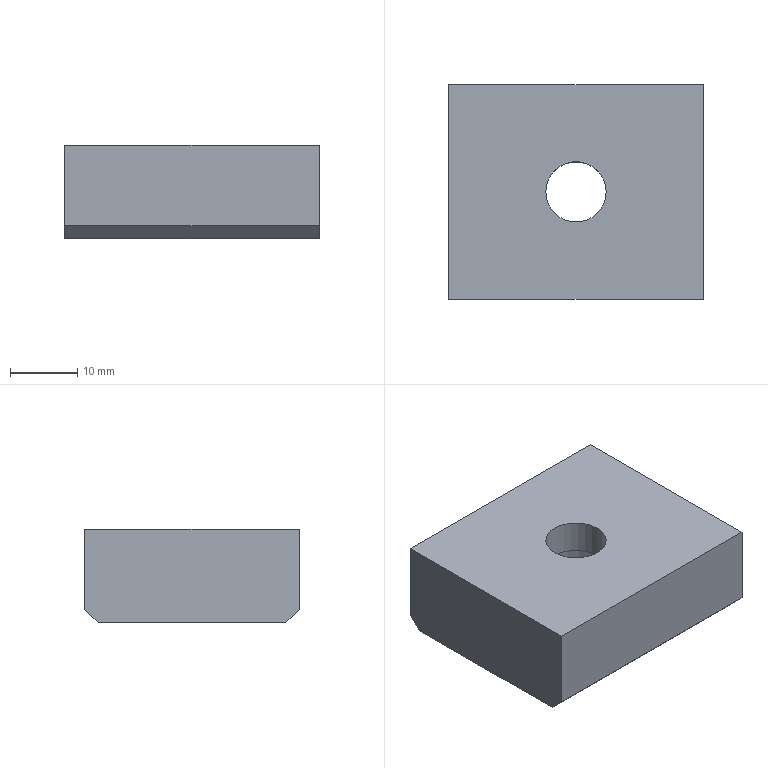Part | NX | features solid 2 | 1 solid | 11 faces | box 38 x 32 x 14 mm | volume 15168 mm3 | plane 9 | cylinder 2 | commonest cylinder face diameters 9 x1 14 x1
STEP:
#1=CARTESIAN_POINT('',(204.,-294.,102.));
#2=VERTEX_POINT('',#1);
#3=CARTESIAN_POINT('',(204.,-294.,114.));
#4=VERTEX_POINT('',#3);
#5=CARTESIAN_POINT('',(204.,-294.,100.));
#6=DIRECTION('',(0.,0.,1.));
#7=VECTOR('',#6,1000.);
#8=LINE('',#5,#7);
#9=EDGE_CURVE('',#2,#4,#8,.T.);
#10=ORIENTED_EDGE('',*,*,#9,.F.);
#11=CARTESIAN_POINT('',(166.,-294.,102.));
#12=VERTEX_POINT('',#11);
#13=CARTESIAN_POINT('',(160.,-294.,102.));
#14=DIRECTION('',(-1.,0.,0.));
#15=VECTOR('',#14,1000.);
#16=LINE('',#13,#15);
#17=EDGE_CURVE('',#2,#12,#16,.T.);
#18=ORIENTED_EDGE('',*,*,#17,.T.);
#19=CARTESIAN_POINT('',(166.,-294.,114.));
#20=VERTEX_POINT('',#19);
#21=CARTESIAN_POINT('',(166.,-294.,100.));
#22=DIRECTION('',(0.,0.,-1.));
#23=VECTOR('',#22,1000.);
#24=LINE('',#21,#23);
#25=EDGE_CURVE('',#12,#20,#24,.F.);
#26=ORIENTED_EDGE('',*,*,#25,.T.);
#27=CARTESIAN_POINT('',(160.,-294.,114.));
#28=DIRECTION('',(-1.,0.,0.));
#29=VECTOR('',#28,1000.);
#30=LINE('',#27,#29);
#31=EDGE_CURVE('',#20,#4,#30,.F.);
#32=ORIENTED_EDGE('',*,*,#31,.T.);
#33=EDGE_LOOP('',(#10,#18,#26,#32));
#34=FACE_BOUND('',#33,.T.);
#35=CARTESIAN_POINT('',(160.,-294.,100.));
#36=DIRECTION('',(0.,1.,0.));
#37=DIRECTION('',(1.,0.,0.));
#38=AXIS2_PLACEMENT_3D('',#35,#36,#37);
#39=PLANE('',#38);
#40=ADVANCED_FACE('',(#34),#39,.T.);
#41=ORIENTED_EDGE('',*,*,#25,.F.);
#42=CARTESIAN_POINT('',(166.,-296.,100.));
#43=VERTEX_POINT('',#42);
#44=CARTESIAN_POINT('',(166.,-298.,98.));
#45=DIRECTION('',(0.,-0.7071,-0.7071));
#46=VECTOR('',#45,1000.);
#47=LINE('',#44,#46);
#48=EDGE_CURVE('',#12,#43,#47,.T.);
#49=ORIENTED_EDGE('',*,*,#48,.T.);
#50=CARTESIAN_POINT('',(166.,-324.,100.));
#51=VERTEX_POINT('',#50);
#52=CARTESIAN_POINT('',(166.,-300.,100.));
#53=DIRECTION('',(0.,1.,0.));
#54=VECTOR('',#53,1000.);
#55=LINE('',#52,#54);
#56=EDGE_CURVE('',#43,#51,#55,.F.);
#57=ORIENTED_EDGE('',*,*,#56,.T.);
#58=CARTESIAN_POINT('',(166.,-326.,102.));
#59=VERTEX_POINT('',#58);
#60=CARTESIAN_POINT('',(166.,-312.,88.));
#61=DIRECTION('',(0.,0.7071,-0.7071));
#62=VECTOR('',#61,1000.);
#63=LINE('',#60,#62);
#64=EDGE_CURVE('',#51,#59,#63,.F.);
#65=ORIENTED_EDGE('',*,*,#64,.T.);
#66=CARTESIAN_POINT('',(166.,-326.,114.));
#67=VERTEX_POINT('',#66);
#68=CARTESIAN_POINT('',(166.,-326.,100.));
#69=DIRECTION('',(0.,0.,1.));
#70=VECTOR('',#69,1000.);
#71=LINE('',#68,#70);
#72=EDGE_CURVE('',#59,#67,#71,.T.);
#73=ORIENTED_EDGE('',*,*,#72,.T.);
#74=CARTESIAN_POINT('',(166.,-300.,114.));
#75=DIRECTION('',(0.,1.,0.));
#76=VECTOR('',#75,1000.);
#77=LINE('',#74,#76);
#78=EDGE_CURVE('',#20,#67,#77,.F.);
#79=ORIENTED_EDGE('',*,*,#78,.F.);
#80=EDGE_LOOP('',(#41,#49,#57,#65,#73,#79));
#81=FACE_BOUND('',#80,.T.);
#82=CARTESIAN_POINT('',(166.,-300.,100.));
#83=DIRECTION('',(1.,0.,0.));
#84=DIRECTION('',(0.,-1.,0.));
#85=AXIS2_PLACEMENT_3D('',#82,#83,#84);
#86=PLANE('',#85);
#87=ADVANCED_FACE('',(#81),#86,.F.);
#88=ORIENTED_EDGE('',*,*,#72,.F.);
#89=CARTESIAN_POINT('',(204.,-326.,102.));
#90=VERTEX_POINT('',#89);
#91=CARTESIAN_POINT('',(160.,-326.,102.));
#92=DIRECTION('',(-1.,0.,0.));
#93=VECTOR('',#92,1000.);
#94=LINE('',#91,#93);
#95=EDGE_CURVE('',#59,#90,#94,.F.);
#96=ORIENTED_EDGE('',*,*,#95,.T.);
#97=CARTESIAN_POINT('',(204.,-326.,114.));
#98=VERTEX_POINT('',#97);
#99=CARTESIAN_POINT('',(204.,-326.,100.));
#100=DIRECTION('',(0.,0.,-1.));
#101=VECTOR('',#100,1000.);
#102=LINE('',#99,#101);
#103=EDGE_CURVE('',#90,#98,#102,.F.);
#104=ORIENTED_EDGE('',*,*,#103,.T.);
#105=CARTESIAN_POINT('',(160.,-326.,114.));
#106=DIRECTION('',(-1.,0.,0.));
#107=VECTOR('',#106,1000.);
#108=LINE('',#105,#107);
#109=EDGE_CURVE('',#67,#98,#108,.F.);
#110=ORIENTED_EDGE('',*,*,#109,.F.);
#111=EDGE_LOOP('',(#88,#96,#104,#110));
#112=FACE_BOUND('',#111,.T.);
#113=CARTESIAN_POINT('',(160.,-326.,100.));
#114=DIRECTION('',(0.,1.,0.));
#115=DIRECTION('',(1.,0.,0.));
#116=AXIS2_PLACEMENT_3D('',#113,#114,#115);
#117=PLANE('',#116);
#118=ADVANCED_FACE('',(#112),#117,.F.);
#119=CARTESIAN_POINT('',(180.5,-310.,114.));
#120=VERTEX_POINT('',#119);
#121=CARTESIAN_POINT('',(185.,-310.,114.));
#122=DIRECTION('',(0.,0.,-1.));
#123=DIRECTION('',(-1.,0.,0.));
#124=AXIS2_PLACEMENT_3D('',#121,#122,#123);
#125=CIRCLE('',#124,4.5);
#126=EDGE_CURVE('',#120,#120,#125,.T.);
#127=ORIENTED_EDGE('',*,*,#126,.T.);
#128=EDGE_LOOP('',(#127));
#129=FACE_BOUND('',#128,.T.);
#130=ORIENTED_EDGE('',*,*,#109,.T.);
#131=CARTESIAN_POINT('',(204.,-300.,114.));
#132=DIRECTION('',(0.,-1.,0.));
#133=VECTOR('',#132,1000.);
#134=LINE('',#131,#133);
#135=EDGE_CURVE('',#4,#98,#134,.T.);
#136=ORIENTED_EDGE('',*,*,#135,.F.);
#137=ORIENTED_EDGE('',*,*,#31,.F.);
#138=ORIENTED_EDGE('',*,*,#78,.T.);
#139=EDGE_LOOP('',(#130,#136,#137,#138));
#140=FACE_BOUND('',#139,.T.);
#141=CARTESIAN_POINT('',(160.,-300.,114.));
#142=DIRECTION('',(0.,0.,-1.));
#143=DIRECTION('',(-1.,0.,0.));
#144=AXIS2_PLACEMENT_3D('',#141,#142,#143);
#145=PLANE('',#144);
#146=ADVANCED_FACE('',(#129,#140),#145,.F.);
#147=CARTESIAN_POINT('',(204.,-296.,100.));
#148=VERTEX_POINT('',#147);
#149=CARTESIAN_POINT('',(204.,-324.,100.));
#150=VERTEX_POINT('',#149);
#151=CARTESIAN_POINT('',(204.,-300.,100.));
#152=DIRECTION('',(0.,-1.,0.));
#153=VECTOR('',#152,1000.);
#154=LINE('',#151,#153);
#155=EDGE_CURVE('',#148,#150,#154,.T.);
#156=ORIENTED_EDGE('',*,*,#155,.F.);
#157=CARTESIAN_POINT('',(204.,-298.,98.));
#158=DIRECTION('',(0.,-0.7071,-0.7071));
#159=VECTOR('',#158,1000.);
#160=LINE('',#157,#159);
#161=EDGE_CURVE('',#148,#2,#160,.F.);
#162=ORIENTED_EDGE('',*,*,#161,.T.);
#163=ORIENTED_EDGE('',*,*,#9,.T.);
#164=ORIENTED_EDGE('',*,*,#135,.T.);
#165=ORIENTED_EDGE('',*,*,#103,.F.);
#166=CARTESIAN_POINT('',(204.,-312.,88.));
#167=DIRECTION('',(0.,0.7071,-0.7071));
#168=VECTOR('',#167,1000.);
#169=LINE('',#166,#168);
#170=EDGE_CURVE('',#90,#150,#169,.T.);
#171=ORIENTED_EDGE('',*,*,#170,.T.);
#172=EDGE_LOOP('',(#156,#162,#163,#164,#165,#171));
#173=FACE_BOUND('',#172,.T.);
#174=CARTESIAN_POINT('',(204.,-300.,100.));
#175=DIRECTION('',(1.,0.,0.));
#176=DIRECTION('',(0.,-1.,0.));
#177=AXIS2_PLACEMENT_3D('',#174,#175,#176);
#178=PLANE('',#177);
#179=ADVANCED_FACE('',(#173),#178,.T.);
#180=CARTESIAN_POINT('',(192.,-310.,100.));
#181=VERTEX_POINT('',#180);
#182=CARTESIAN_POINT('',(185.,-310.,100.));
#183=DIRECTION('',(0.,0.,1.));
#184=DIRECTION('',(1.,0.,0.));
#185=AXIS2_PLACEMENT_3D('',#182,#183,#184);
#186=CIRCLE('',#185,7.);
#187=EDGE_CURVE('',#181,#181,#186,.T.);
#188=ORIENTED_EDGE('',*,*,#187,.T.);
#189=EDGE_LOOP('',(#188));
#190=FACE_BOUND('',#189,.T.);
#191=ORIENTED_EDGE('',*,*,#56,.F.);
#192=CARTESIAN_POINT('',(160.,-296.,100.));
#193=DIRECTION('',(1.,0.,0.));
#194=VECTOR('',#193,1000.);
#195=LINE('',#192,#194);
#196=EDGE_CURVE('',#43,#148,#195,.T.);
#197=ORIENTED_EDGE('',*,*,#196,.T.);
#198=ORIENTED_EDGE('',*,*,#155,.T.);
#199=CARTESIAN_POINT('',(160.,-324.,100.));
#200=DIRECTION('',(-1.,0.,0.));
#201=VECTOR('',#200,1000.);
#202=LINE('',#199,#201);
#203=EDGE_CURVE('',#150,#51,#202,.T.);
#204=ORIENTED_EDGE('',*,*,#203,.T.);
#205=EDGE_LOOP('',(#191,#197,#198,#204));
#206=FACE_BOUND('',#205,.T.);
#207=CARTESIAN_POINT('',(160.,-300.,100.));
#208=DIRECTION('',(0.,0.,-1.));
#209=DIRECTION('',(-1.,0.,0.));
#210=AXIS2_PLACEMENT_3D('',#207,#208,#209);
#211=PLANE('',#210);
#212=ADVANCED_FACE('',(#190,#206),#211,.T.);
#213=ORIENTED_EDGE('',*,*,#48,.F.);
#214=ORIENTED_EDGE('',*,*,#17,.F.);
#215=ORIENTED_EDGE('',*,*,#161,.F.);
#216=ORIENTED_EDGE('',*,*,#196,.F.);
#217=EDGE_LOOP('',(#213,#214,#215,#216));
#218=FACE_BOUND('',#217,.T.);
#219=CARTESIAN_POINT('',(160.,-296.,100.));
#220=DIRECTION('',(0.,-0.7071,0.7071));
#221=DIRECTION('',(0.,-0.7071,-0.7071));
#222=AXIS2_PLACEMENT_3D('',#219,#220,#221);
#223=PLANE('',#222);
#224=ADVANCED_FACE('',(#218),#223,.F.);
#225=ORIENTED_EDGE('',*,*,#64,.F.);
#226=ORIENTED_EDGE('',*,*,#203,.F.);
#227=ORIENTED_EDGE('',*,*,#170,.F.);
#228=ORIENTED_EDGE('',*,*,#95,.F.);
#229=EDGE_LOOP('',(#225,#226,#227,#228));
#230=FACE_BOUND('',#229,.T.);
#231=CARTESIAN_POINT('',(160.,-326.,102.));
#232=DIRECTION('',(0.,-0.7071,-0.7071));
#233=DIRECTION('',(0.,0.7071,-0.7071));
#234=AXIS2_PLACEMENT_3D('',#231,#232,#233);
#235=PLANE('',#234);
#236=ADVANCED_FACE('',(#230),#235,.T.);
#237=ORIENTED_EDGE('',*,*,#187,.F.);
#238=EDGE_LOOP('',(#237));
#239=FACE_BOUND('',#238,.T.);
#240=CARTESIAN_POINT('',(192.,-310.,109.));
#241=VERTEX_POINT('',#240);
#242=CARTESIAN_POINT('',(185.,-310.,109.));
#243=DIRECTION('',(0.,0.,1.));
#244=DIRECTION('',(1.,0.,0.));
#245=AXIS2_PLACEMENT_3D('',#242,#243,#244);
#246=CIRCLE('',#245,7.);
#247=EDGE_CURVE('',#241,#241,#246,.T.);
#248=ORIENTED_EDGE('',*,*,#247,.T.);
#249=EDGE_LOOP('',(#248));
#250=FACE_BOUND('',#249,.T.);
#251=CARTESIAN_POINT('',(185.,-310.,100.));
#252=DIRECTION('',(0.,0.,1.));
#253=DIRECTION('',(1.,0.,0.));
#254=AXIS2_PLACEMENT_3D('',#251,#252,#253);
#255=CYLINDRICAL_SURFACE('',#254,7.);
#256=ADVANCED_FACE('',(#239,#250),#255,.F.);
#257=CARTESIAN_POINT('',(189.5,-310.,109.));
#258=VERTEX_POINT('',#257);
#259=CARTESIAN_POINT('',(185.,-310.,109.));
#260=DIRECTION('',(0.,0.,1.));
#261=DIRECTION('',(1.,0.,0.));
#262=AXIS2_PLACEMENT_3D('',#259,#260,#261);
#263=CIRCLE('',#262,4.5);
#264=EDGE_CURVE('',#258,#258,#263,.T.);
#265=ORIENTED_EDGE('',*,*,#264,.T.);
#266=EDGE_LOOP('',(#265));
#267=FACE_BOUND('',#266,.T.);
#268=ORIENTED_EDGE('',*,*,#247,.F.);
#269=EDGE_LOOP('',(#268));
#270=FACE_BOUND('',#269,.T.);
#271=CARTESIAN_POINT('',(185.,-310.,109.));
#272=DIRECTION('',(0.,0.,1.));
#273=DIRECTION('',(1.,0.,0.));
#274=AXIS2_PLACEMENT_3D('',#271,#272,#273);
#275=PLANE('',#274);
#276=ADVANCED_FACE('',(#267,#270),#275,.F.);
#277=ORIENTED_EDGE('',*,*,#264,.F.);
#278=EDGE_LOOP('',(#277));
#279=FACE_BOUND('',#278,.T.);
#280=ORIENTED_EDGE('',*,*,#126,.F.);
#281=EDGE_LOOP('',(#280));
#282=FACE_BOUND('',#281,.T.);
#283=CARTESIAN_POINT('',(185.,-310.,100.));
#284=DIRECTION('',(0.,0.,1.));
#285=DIRECTION('',(1.,0.,0.));
#286=AXIS2_PLACEMENT_3D('',#283,#284,#285);
#287=CYLINDRICAL_SURFACE('',#286,4.5);
#288=ADVANCED_FACE('',(#279,#282),#287,.F.);
#289=CLOSED_SHELL('',(#40,#87,#118,#146,#179,#212,#224,#236,#256,#276,#288));
#290=MANIFOLD_SOLID_BREP('',#289);
#291=(LENGTH_UNIT()NAMED_UNIT(*)SI_UNIT(.MILLI.,.METRE.));
#292=UNCERTAINTY_MEASURE_WITH_UNIT(LENGTH_MEASURE(0.00001),#291,'','');
#293=(NAMED_UNIT(*)PLANE_ANGLE_UNIT()SI_UNIT($,.RADIAN.));
#294=(NAMED_UNIT(*)SI_UNIT($,.STERADIAN.)SOLID_ANGLE_UNIT());
#295=(GEOMETRIC_REPRESENTATION_CONTEXT(3)GLOBAL_UNCERTAINTY_ASSIGNED_CONTEXT((#292))GLOBAL_UNIT_ASSIGNED_CONTEXT((#291,#293,#294))REPRESENTATION_CONTEXT('',''));
#296=ADVANCED_BREP_SHAPE_REPRESENTATION('',(#290),#295);